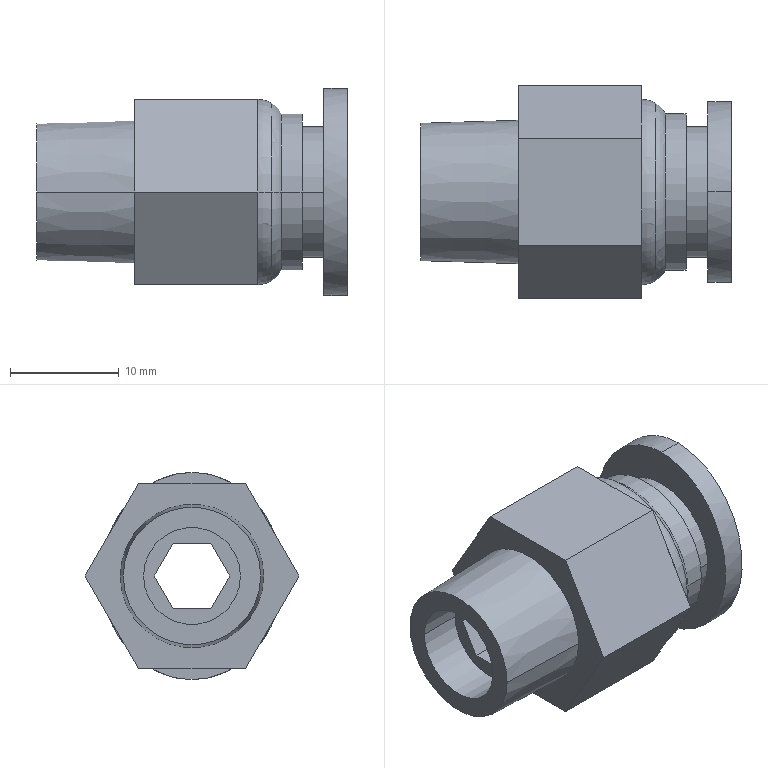Part | Creo | 1 solid | 45 faces | box 28.5 x 19.63 x 19 mm | volume 3530 mm3 | plane 25 | cylinder 8 | torus 8 | cone 2 | other 2 | commonest cylinder face diameters 8.9 x2 10 x2 12 x2 14.36 x2
STEP:
#1=CARTESIAN_POINT('',(308.,140.545,-32.491));
#2=VERTEX_POINT('',#1);
#3=CARTESIAN_POINT('',(308.,149.445,-32.491));
#4=VERTEX_POINT('',#3);
#5=CARTESIAN_POINT('',(308.,144.995,-32.491));
#6=DIRECTION('',(-1.,0.,0.));
#7=DIRECTION('',(0.,-1.,0.));
#8=AXIS2_PLACEMENT_3D('',#5,#6,#7);
#9=CIRCLE('',#8,4.45);
#10=EDGE_CURVE('',#2,#4,#9,.T.);
#11=ORIENTED_EDGE('',*,*,#10,.F.);
#12=CARTESIAN_POINT('',(308.,144.995,-32.491));
#13=DIRECTION('',(-1.,0.,0.));
#14=DIRECTION('',(0.,1.,0.));
#15=AXIS2_PLACEMENT_3D('',#12,#13,#14);
#16=CIRCLE('',#15,4.45);
#17=EDGE_CURVE('',#4,#2,#16,.T.);
#18=ORIENTED_EDGE('',*,*,#17,.F.);
#19=EDGE_LOOP('',(#11,#18));
#20=FACE_OUTER_BOUND('',#19,.F.);
#21=CARTESIAN_POINT('',(308.,146.727,-35.491));
#22=VERTEX_POINT('',#21);
#23=CARTESIAN_POINT('',(308.,148.459,-32.491));
#24=VERTEX_POINT('',#23);
#25=CARTESIAN_POINT('',(308.,146.727,-35.491));
#26=DIRECTION('',(0.,0.5,0.866));
#27=VECTOR('',#26,3.464);
#28=LINE('',#25,#27);
#29=EDGE_CURVE('',#22,#24,#28,.T.);
#30=ORIENTED_EDGE('',*,*,#29,.F.);
#31=CARTESIAN_POINT('',(308.,143.263,-35.491));
#32=VERTEX_POINT('',#31);
#33=CARTESIAN_POINT('',(308.,143.263,-35.491));
#34=DIRECTION('',(0.,1.,0.));
#35=VECTOR('',#34,3.464);
#36=LINE('',#33,#35);
#37=EDGE_CURVE('',#32,#22,#36,.T.);
#38=ORIENTED_EDGE('',*,*,#37,.F.);
#39=CARTESIAN_POINT('',(308.,141.531,-32.491));
#40=VERTEX_POINT('',#39);
#41=CARTESIAN_POINT('',(308.,141.531,-32.491));
#42=DIRECTION('',(0.,0.5,-0.866));
#43=VECTOR('',#42,3.464);
#44=LINE('',#41,#43);
#45=EDGE_CURVE('',#40,#32,#44,.T.);
#46=ORIENTED_EDGE('',*,*,#45,.F.);
#47=CARTESIAN_POINT('',(308.,143.263,-29.491));
#48=VERTEX_POINT('',#47);
#49=CARTESIAN_POINT('',(308.,143.263,-29.491));
#50=DIRECTION('',(0.,-0.5,-0.866));
#51=VECTOR('',#50,3.464);
#52=LINE('',#49,#51);
#53=EDGE_CURVE('',#48,#40,#52,.T.);
#54=ORIENTED_EDGE('',*,*,#53,.F.);
#55=CARTESIAN_POINT('',(308.,146.727,-29.491));
#56=VERTEX_POINT('',#55);
#57=CARTESIAN_POINT('',(308.,146.727,-29.491));
#58=DIRECTION('',(0.,-1.,0.));
#59=VECTOR('',#58,3.464);
#60=LINE('',#57,#59);
#61=EDGE_CURVE('',#56,#48,#60,.T.);
#62=ORIENTED_EDGE('',*,*,#61,.F.);
#63=CARTESIAN_POINT('',(308.,148.459,-32.491));
#64=DIRECTION('',(0.,-0.5,0.866));
#65=VECTOR('',#64,3.464);
#66=LINE('',#63,#65);
#67=EDGE_CURVE('',#24,#56,#66,.T.);
#68=ORIENTED_EDGE('',*,*,#67,.F.);
#69=EDGE_LOOP('',(#30,#38,#46,#54,#62,#68));
#70=FACE_BOUND('',#69,.F.);
#71=CARTESIAN_POINT('',(308.,144.995,-28.041));
#72=DIRECTION('',(1.,0.,0.));
#73=DIRECTION('',(0.,1.,0.));
#74=AXIS2_PLACEMENT_3D('',#71,#72,#73);
#75=PLANE('',#74);
#76=ADVANCED_FACE('',(#20,#70),#75,.F.);
#77=CARTESIAN_POINT('',(304.,149.445,-32.491));
#78=VERTEX_POINT('',#77);
#79=CARTESIAN_POINT('',(304.,140.545,-32.491));
#80=VERTEX_POINT('',#79);
#81=CARTESIAN_POINT('',(304.,144.995,-32.491));
#82=DIRECTION('',(1.,0.,0.));
#83=DIRECTION('',(0.,1.,0.));
#84=AXIS2_PLACEMENT_3D('',#81,#82,#83);
#85=CIRCLE('',#84,4.45);
#86=EDGE_CURVE('',#78,#80,#85,.T.);
#87=ORIENTED_EDGE('',*,*,#86,.T.);
#88=CARTESIAN_POINT('',(308.,140.545,-32.491));
#89=DIRECTION('',(-1.,0.,0.));
#90=VECTOR('',#89,4.);
#91=LINE('',#88,#90);
#92=EDGE_CURVE('',#2,#80,#91,.T.);
#93=ORIENTED_EDGE('',*,*,#92,.F.);
#94=ORIENTED_EDGE('',*,*,#10,.T.);
#95=CARTESIAN_POINT('',(308.,149.445,-32.491));
#96=DIRECTION('',(-1.,0.,0.));
#97=VECTOR('',#96,4.);
#98=LINE('',#95,#97);
#99=EDGE_CURVE('',#4,#78,#98,.T.);
#100=ORIENTED_EDGE('',*,*,#99,.T.);
#101=EDGE_LOOP('',(#87,#93,#94,#100));
#102=FACE_OUTER_BOUND('',#101,.F.);
#103=CARTESIAN_POINT('',(335.,144.995,-32.491));
#104=DIRECTION('',(-1.,0.,0.));
#105=DIRECTION('',(0.,-1.,0.));
#106=AXIS2_PLACEMENT_3D('',#103,#104,#105);
#107=CYLINDRICAL_SURFACE('',#106,4.45);
#108=ADVANCED_FACE('',(#102),#107,.F.);
#109=CARTESIAN_POINT('',(304.,151.296,-32.491));
#110=VERTEX_POINT('',#109);
#111=CARTESIAN_POINT('',(304.,138.694,-32.491));
#112=VERTEX_POINT('',#111);
#113=CARTESIAN_POINT('',(304.,144.995,-32.491));
#114=DIRECTION('',(-1.,0.,0.));
#115=DIRECTION('',(0.,1.,0.));
#116=AXIS2_PLACEMENT_3D('',#113,#114,#115);
#117=CIRCLE('',#116,6.301);
#118=EDGE_CURVE('',#110,#112,#117,.T.);
#119=ORIENTED_EDGE('',*,*,#118,.F.);
#120=CARTESIAN_POINT('',(304.,144.995,-32.491));
#121=DIRECTION('',(-1.,0.,0.));
#122=DIRECTION('',(0.,-1.,0.));
#123=AXIS2_PLACEMENT_3D('',#120,#121,#122);
#124=CIRCLE('',#123,6.301);
#125=EDGE_CURVE('',#112,#110,#124,.T.);
#126=ORIENTED_EDGE('',*,*,#125,.F.);
#127=EDGE_LOOP('',(#119,#126));
#128=FACE_OUTER_BOUND('',#127,.F.);
#129=CARTESIAN_POINT('',(304.,144.995,-32.491));
#130=DIRECTION('',(1.,0.,0.));
#131=DIRECTION('',(0.,-1.,0.));
#132=AXIS2_PLACEMENT_3D('',#129,#130,#131);
#133=CIRCLE('',#132,4.45);
#134=EDGE_CURVE('',#80,#78,#133,.T.);
#135=ORIENTED_EDGE('',*,*,#134,.F.);
#136=ORIENTED_EDGE('',*,*,#86,.F.);
#137=EDGE_LOOP('',(#135,#136));
#138=FACE_BOUND('',#137,.F.);
#139=CARTESIAN_POINT('',(304.,144.995,-26.19));
#140=DIRECTION('',(-1.,0.,0.));
#141=DIRECTION('',(0.,-1.,0.));
#142=AXIS2_PLACEMENT_3D('',#139,#140,#141);
#143=PLANE('',#142);
#144=ADVANCED_FACE('',(#128,#138),#143,.T.);
#145=ORIENTED_EDGE('',*,*,#134,.T.);
#146=ORIENTED_EDGE('',*,*,#99,.F.);
#147=ORIENTED_EDGE('',*,*,#17,.T.);
#148=ORIENTED_EDGE('',*,*,#92,.T.);
#149=EDGE_LOOP('',(#145,#146,#147,#148));
#150=FACE_OUTER_BOUND('',#149,.F.);
#151=CARTESIAN_POINT('',(335.,144.995,-32.491));
#152=DIRECTION('',(-1.,0.,0.));
#153=DIRECTION('',(0.,-1.,0.));
#154=AXIS2_PLACEMENT_3D('',#151,#152,#153);
#155=CYLINDRICAL_SURFACE('',#154,4.45);
#156=ADVANCED_FACE('',(#150),#155,.F.);
#157=ORIENTED_EDGE('',*,*,#118,.T.);
#158=CARTESIAN_POINT('',(313.,138.415,-32.491));
#159=VERTEX_POINT('',#158);
#160=CARTESIAN_POINT('',(304.,138.694,-32.491));
#161=DIRECTION('',(0.9995,-0.03097,0.));
#162=VECTOR('',#161,9.004);
#163=LINE('',#160,#162);
#164=EDGE_CURVE('',#112,#159,#163,.T.);
#165=ORIENTED_EDGE('',*,*,#164,.T.);
#166=CARTESIAN_POINT('',(313.,151.575,-32.491));
#167=VERTEX_POINT('',#166);
#168=CARTESIAN_POINT('',(313.,144.995,-32.491));
#169=DIRECTION('',(1.,0.,0.));
#170=DIRECTION('',(0.,-1.,0.));
#171=AXIS2_PLACEMENT_3D('',#168,#169,#170);
#172=CIRCLE('',#171,6.58);
#173=EDGE_CURVE('',#159,#167,#172,.T.);
#174=ORIENTED_EDGE('',*,*,#173,.T.);
#175=CARTESIAN_POINT('',(304.,151.296,-32.491));
#176=DIRECTION('',(0.9995,0.03097,0.));
#177=VECTOR('',#176,9.004);
#178=LINE('',#175,#177);
#179=EDGE_CURVE('',#110,#167,#178,.T.);
#180=ORIENTED_EDGE('',*,*,#179,.F.);
#181=EDGE_LOOP('',(#157,#165,#174,#180));
#182=FACE_OUTER_BOUND('',#181,.F.);
#183=CARTESIAN_POINT('',(308.5,144.995,-32.491));
#184=DIRECTION('',(1.,0.,0.));
#185=DIRECTION('',(0.,1.,0.));
#186=AXIS2_PLACEMENT_3D('',#183,#184,#185);
#187=CONICAL_SURFACE('',#186,6.441,1.775);
#188=ADVANCED_FACE('',(#182),#187,.T.);
#189=ORIENTED_EDGE('',*,*,#125,.T.);
#190=ORIENTED_EDGE('',*,*,#179,.T.);
#191=CARTESIAN_POINT('',(313.,144.995,-32.491));
#192=DIRECTION('',(1.,0.,0.));
#193=DIRECTION('',(0.,1.,0.));
#194=AXIS2_PLACEMENT_3D('',#191,#192,#193);
#195=CIRCLE('',#194,6.58);
#196=EDGE_CURVE('',#167,#159,#195,.T.);
#197=ORIENTED_EDGE('',*,*,#196,.T.);
#198=ORIENTED_EDGE('',*,*,#164,.F.);
#199=EDGE_LOOP('',(#189,#190,#197,#198));
#200=FACE_OUTER_BOUND('',#199,.F.);
#201=CARTESIAN_POINT('',(308.5,144.995,-32.491));
#202=DIRECTION('',(1.,0.,0.));
#203=DIRECTION('',(0.,1.,0.));
#204=AXIS2_PLACEMENT_3D('',#201,#202,#203);
#205=CONICAL_SURFACE('',#204,6.441,1.775);
#206=ADVANCED_FACE('',(#200),#205,.T.);
#207=CARTESIAN_POINT('',(313.,135.18,-32.491));
#208=VERTEX_POINT('',#207);
#209=CARTESIAN_POINT('',(313.,140.088,-23.991));
#210=VERTEX_POINT('',#209);
#211=CARTESIAN_POINT('',(313.,135.18,-32.491));
#212=DIRECTION('',(0.,0.5,0.866));
#213=VECTOR('',#212,9.815);
#214=LINE('',#211,#213);
#215=EDGE_CURVE('',#208,#210,#214,.T.);
#216=ORIENTED_EDGE('',*,*,#215,.F.);
#217=CARTESIAN_POINT('',(313.,140.088,-40.991));
#218=VERTEX_POINT('',#217);
#219=CARTESIAN_POINT('',(313.,140.088,-40.991));
#220=DIRECTION('',(0.,-0.5,0.866));
#221=VECTOR('',#220,9.815);
#222=LINE('',#219,#221);
#223=EDGE_CURVE('',#218,#208,#222,.T.);
#224=ORIENTED_EDGE('',*,*,#223,.F.);
#225=CARTESIAN_POINT('',(313.,149.903,-40.991));
#226=VERTEX_POINT('',#225);
#227=CARTESIAN_POINT('',(313.,140.088,-40.991));
#228=DIRECTION('',(0.,1.,0.));
#229=VECTOR('',#228,9.815);
#230=LINE('',#227,#229);
#231=EDGE_CURVE('',#218,#226,#230,.T.);
#232=ORIENTED_EDGE('',*,*,#231,.T.);
#233=CARTESIAN_POINT('',(313.,154.81,-32.491));
#234=VERTEX_POINT('',#233);
#235=CARTESIAN_POINT('',(313.,154.81,-32.491));
#236=DIRECTION('',(0.,-0.5,-0.866));
#237=VECTOR('',#236,9.815);
#238=LINE('',#235,#237);
#239=EDGE_CURVE('',#234,#226,#238,.T.);
#240=ORIENTED_EDGE('',*,*,#239,.F.);
#241=CARTESIAN_POINT('',(313.,149.903,-23.991));
#242=VERTEX_POINT('',#241);
#243=CARTESIAN_POINT('',(313.,149.903,-23.991));
#244=DIRECTION('',(0.,0.5,-0.866));
#245=VECTOR('',#244,9.815);
#246=LINE('',#243,#245);
#247=EDGE_CURVE('',#242,#234,#246,.T.);
#248=ORIENTED_EDGE('',*,*,#247,.F.);
#249=CARTESIAN_POINT('',(313.,149.903,-23.991));
#250=DIRECTION('',(0.,-1.,0.));
#251=VECTOR('',#250,9.815);
#252=LINE('',#249,#251);
#253=EDGE_CURVE('',#242,#210,#252,.T.);
#254=ORIENTED_EDGE('',*,*,#253,.T.);
#255=EDGE_LOOP('',(#216,#224,#232,#240,#248,#254));
#256=FACE_OUTER_BOUND('',#255,.F.);
#257=ORIENTED_EDGE('',*,*,#196,.F.);
#258=ORIENTED_EDGE('',*,*,#173,.F.);
#259=EDGE_LOOP('',(#257,#258));
#260=FACE_BOUND('',#259,.F.);
#261=CARTESIAN_POINT('',(313.,144.995,-25.841));
#262=DIRECTION('',(-1.,0.,0.));
#263=DIRECTION('',(0.,-1.,0.));
#264=AXIS2_PLACEMENT_3D('',#261,#262,#263);
#265=PLANE('',#264);
#266=ADVANCED_FACE('',(#256,#260),#265,.T.);
#267=ORIENTED_EDGE('',*,*,#215,.T.);
#268=CARTESIAN_POINT('',(324.3,140.088,-23.991));
#269=VERTEX_POINT('',#268);
#270=CARTESIAN_POINT('',(313.,140.088,-23.991));
#271=DIRECTION('',(1.,0.,0.));
#272=VECTOR('',#271,11.3);
#273=LINE('',#270,#272);
#274=EDGE_CURVE('',#210,#269,#273,.T.);
#275=ORIENTED_EDGE('',*,*,#274,.T.);
#276=CARTESIAN_POINT('',(324.3,137.634,-28.241));
#277=VERTEX_POINT('',#276);
#278=CARTESIAN_POINT('',(324.3,140.088,-23.991));
#279=DIRECTION('',(0.,-0.5,-0.866));
#280=VECTOR('',#279,4.907);
#281=LINE('',#278,#280);
#282=EDGE_CURVE('',#269,#277,#281,.T.);
#283=ORIENTED_EDGE('',*,*,#282,.T.);
#284=CARTESIAN_POINT('',(324.3,135.18,-32.491));
#285=VERTEX_POINT('',#284);
#286=CARTESIAN_POINT('',(324.3,137.634,-28.241));
#287=DIRECTION('',(0.,-0.5,-0.866));
#288=VECTOR('',#287,4.907);
#289=LINE('',#286,#288);
#290=EDGE_CURVE('',#277,#285,#289,.T.);
#291=ORIENTED_EDGE('',*,*,#290,.T.);
#292=CARTESIAN_POINT('',(313.,135.18,-32.491));
#293=DIRECTION('',(1.,0.,0.));
#294=VECTOR('',#293,11.3);
#295=LINE('',#292,#294);
#296=EDGE_CURVE('',#208,#285,#295,.T.);
#297=ORIENTED_EDGE('',*,*,#296,.F.);
#298=EDGE_LOOP('',(#267,#275,#283,#291,#297));
#299=FACE_OUTER_BOUND('',#298,.F.);
#300=CARTESIAN_POINT('',(324.3,135.18,-32.491));
#301=DIRECTION('',(0.,-0.866,0.5));
#302=DIRECTION('',(0.,-0.5,-0.866));
#303=AXIS2_PLACEMENT_3D('',#300,#301,#302);
#304=PLANE('',#303);
#305=ADVANCED_FACE('',(#299),#304,.T.);
#306=ORIENTED_EDGE('',*,*,#253,.F.);
#307=CARTESIAN_POINT('',(324.3,149.903,-23.991));
#308=VERTEX_POINT('',#307);
#309=CARTESIAN_POINT('',(313.,149.903,-23.991));
#310=DIRECTION('',(1.,0.,0.));
#311=VECTOR('',#310,11.3);
#312=LINE('',#309,#311);
#313=EDGE_CURVE('',#242,#308,#312,.T.);
#314=ORIENTED_EDGE('',*,*,#313,.T.);
#315=CARTESIAN_POINT('',(324.3,144.995,-23.991));
#316=VERTEX_POINT('',#315);
#317=CARTESIAN_POINT('',(324.3,149.903,-23.991));
#318=DIRECTION('',(0.,-1.,0.));
#319=VECTOR('',#318,4.907);
#320=LINE('',#317,#319);
#321=EDGE_CURVE('',#308,#316,#320,.T.);
#322=ORIENTED_EDGE('',*,*,#321,.T.);
#323=CARTESIAN_POINT('',(324.3,144.995,-23.991));
#324=DIRECTION('',(0.,-1.,0.));
#325=VECTOR('',#324,4.907);
#326=LINE('',#323,#325);
#327=EDGE_CURVE('',#316,#269,#326,.T.);
#328=ORIENTED_EDGE('',*,*,#327,.T.);
#329=ORIENTED_EDGE('',*,*,#274,.F.);
#330=EDGE_LOOP('',(#306,#314,#322,#328,#329));
#331=FACE_OUTER_BOUND('',#330,.F.);
#332=CARTESIAN_POINT('',(324.3,140.088,-23.991));
#333=DIRECTION('',(0.,0.,1.));
#334=DIRECTION('',(1.,0.,0.));
#335=AXIS2_PLACEMENT_3D('',#332,#333,#334);
#336=PLANE('',#335);
#337=ADVANCED_FACE('',(#331),#336,.T.);
#338=CARTESIAN_POINT('',(324.3,154.81,-32.491));
#339=VERTEX_POINT('',#338);
#340=CARTESIAN_POINT('',(313.,154.81,-32.491));
#341=DIRECTION('',(1.,0.,0.));
#342=VECTOR('',#341,11.3);
#343=LINE('',#340,#342);
#344=EDGE_CURVE('',#234,#339,#343,.T.);
#345=ORIENTED_EDGE('',*,*,#344,.T.);
#346=CARTESIAN_POINT('',(324.3,152.357,-28.241));
#347=VERTEX_POINT('',#346);
#348=CARTESIAN_POINT('',(324.3,154.81,-32.491));
#349=DIRECTION('',(0.,-0.5,0.866));
#350=VECTOR('',#349,4.907);
#351=LINE('',#348,#350);
#352=EDGE_CURVE('',#339,#347,#351,.T.);
#353=ORIENTED_EDGE('',*,*,#352,.T.);
#354=CARTESIAN_POINT('',(324.3,152.357,-28.241));
#355=DIRECTION('',(0.,-0.5,0.866));
#356=VECTOR('',#355,4.907);
#357=LINE('',#354,#356);
#358=EDGE_CURVE('',#347,#308,#357,.T.);
#359=ORIENTED_EDGE('',*,*,#358,.T.);
#360=ORIENTED_EDGE('',*,*,#313,.F.);
#361=ORIENTED_EDGE('',*,*,#247,.T.);
#362=EDGE_LOOP('',(#345,#353,#359,#360,#361));
#363=FACE_OUTER_BOUND('',#362,.F.);
#364=CARTESIAN_POINT('',(324.3,149.903,-23.991));
#365=DIRECTION('',(0.,0.866,0.5));
#366=DIRECTION('',(0.,-0.5,0.866));
#367=AXIS2_PLACEMENT_3D('',#364,#365,#366);
#368=PLANE('',#367);
#369=ADVANCED_FACE('',(#363),#368,.T.);
#370=ORIENTED_EDGE('',*,*,#239,.T.);
#371=CARTESIAN_POINT('',(324.3,149.903,-40.991));
#372=VERTEX_POINT('',#371);
#373=CARTESIAN_POINT('',(313.,149.903,-40.991));
#374=DIRECTION('',(1.,0.,0.));
#375=VECTOR('',#374,11.3);
#376=LINE('',#373,#375);
#377=EDGE_CURVE('',#226,#372,#376,.T.);
#378=ORIENTED_EDGE('',*,*,#377,.T.);
#379=CARTESIAN_POINT('',(324.3,152.357,-36.741));
#380=VERTEX_POINT('',#379);
#381=CARTESIAN_POINT('',(324.3,149.903,-40.991));
#382=DIRECTION('',(0.,0.5,0.866));
#383=VECTOR('',#382,4.907);
#384=LINE('',#381,#383);
#385=EDGE_CURVE('',#372,#380,#384,.T.);
#386=ORIENTED_EDGE('',*,*,#385,.T.);
#387=CARTESIAN_POINT('',(324.3,152.357,-36.741));
#388=DIRECTION('',(0.,0.5,0.866));
#389=VECTOR('',#388,4.907);
#390=LINE('',#387,#389);
#391=EDGE_CURVE('',#380,#339,#390,.T.);
#392=ORIENTED_EDGE('',*,*,#391,.T.);
#393=ORIENTED_EDGE('',*,*,#344,.F.);
#394=EDGE_LOOP('',(#370,#378,#386,#392,#393));
#395=FACE_OUTER_BOUND('',#394,.F.);
#396=CARTESIAN_POINT('',(324.3,154.81,-32.491));
#397=DIRECTION('',(0.,0.866,-0.5));
#398=DIRECTION('',(0.,0.5,0.866));
#399=AXIS2_PLACEMENT_3D('',#396,#397,#398);
#400=PLANE('',#399);
#401=ADVANCED_FACE('',(#395),#400,.T.);
#402=ORIENTED_EDGE('',*,*,#231,.F.);
#403=CARTESIAN_POINT('',(324.3,140.088,-40.991));
#404=VERTEX_POINT('',#403);
#405=CARTESIAN_POINT('',(313.,140.088,-40.991));
#406=DIRECTION('',(1.,0.,0.));
#407=VECTOR('',#406,11.3);
#408=LINE('',#405,#407);
#409=EDGE_CURVE('',#218,#404,#408,.T.);
#410=ORIENTED_EDGE('',*,*,#409,.T.);
#411=CARTESIAN_POINT('',(324.3,144.995,-40.991));
#412=VERTEX_POINT('',#411);
#413=CARTESIAN_POINT('',(324.3,140.088,-40.991));
#414=DIRECTION('',(0.,1.,0.));
#415=VECTOR('',#414,4.907);
#416=LINE('',#413,#415);
#417=EDGE_CURVE('',#404,#412,#416,.T.);
#418=ORIENTED_EDGE('',*,*,#417,.T.);
#419=CARTESIAN_POINT('',(324.3,144.995,-40.991));
#420=DIRECTION('',(0.,1.,0.));
#421=VECTOR('',#420,4.907);
#422=LINE('',#419,#421);
#423=EDGE_CURVE('',#412,#372,#422,.T.);
#424=ORIENTED_EDGE('',*,*,#423,.T.);
#425=ORIENTED_EDGE('',*,*,#377,.F.);
#426=EDGE_LOOP('',(#402,#410,#418,#424,#425));
#427=FACE_OUTER_BOUND('',#426,.F.);
#428=CARTESIAN_POINT('',(324.3,149.903,-40.991));
#429=DIRECTION('',(0.,0.,-1.));
#430=DIRECTION('',(0.,1.,0.));
#431=AXIS2_PLACEMENT_3D('',#428,#429,#430);
#432=PLANE('',#431);
#433=ADVANCED_FACE('',(#427),#432,.T.);
#434=ORIENTED_EDGE('',*,*,#223,.T.);
#435=ORIENTED_EDGE('',*,*,#296,.T.);
#436=CARTESIAN_POINT('',(324.3,137.634,-36.741));
#437=VERTEX_POINT('',#436);
#438=CARTESIAN_POINT('',(324.3,135.18,-32.491));
#439=DIRECTION('',(0.,0.5,-0.866));
#440=VECTOR('',#439,4.907);
#441=LINE('',#438,#440);
#442=EDGE_CURVE('',#285,#437,#441,.T.);
#443=ORIENTED_EDGE('',*,*,#442,.T.);
#444=CARTESIAN_POINT('',(324.3,137.634,-36.741));
#445=DIRECTION('',(0.,0.5,-0.866));
#446=VECTOR('',#445,4.907);
#447=LINE('',#444,#446);
#448=EDGE_CURVE('',#437,#404,#447,.T.);
#449=ORIENTED_EDGE('',*,*,#448,.T.);
#450=ORIENTED_EDGE('',*,*,#409,.F.);
#451=EDGE_LOOP('',(#434,#435,#443,#449,#450));
#452=FACE_OUTER_BOUND('',#451,.F.);
#453=CARTESIAN_POINT('',(324.3,140.088,-40.991));
#454=DIRECTION('',(0.,-0.866,-0.5));
#455=DIRECTION('',(0.,0.5,-0.866));
#456=AXIS2_PLACEMENT_3D('',#453,#454,#455);
#457=PLANE('',#456);
#458=ADVANCED_FACE('',(#452),#457,.T.);
#459=CARTESIAN_POINT('',(324.3,136.495,-32.491));
#460=VERTEX_POINT('',#459);
#461=CARTESIAN_POINT('',(324.3,144.995,-32.491));
#462=DIRECTION('',(-1.,0.,0.));
#463=DIRECTION('',(0.,-0.866,-0.5));
#464=AXIS2_PLACEMENT_3D('',#461,#462,#463);
#465=CIRCLE('',#464,8.5);
#466=EDGE_CURVE('',#437,#460,#465,.T.);
#467=ORIENTED_EDGE('',*,*,#466,.F.);
#468=ORIENTED_EDGE('',*,*,#442,.F.);
#469=ORIENTED_EDGE('',*,*,#290,.F.);
#470=CARTESIAN_POINT('',(324.3,144.995,-32.491));
#471=DIRECTION('',(-1.,0.,0.));
#472=DIRECTION('',(0.,-1.,0.));
#473=AXIS2_PLACEMENT_3D('',#470,#471,#472);
#474=CIRCLE('',#473,8.5);
#475=EDGE_CURVE('',#460,#277,#474,.T.);
#476=ORIENTED_EDGE('',*,*,#475,.F.);
#477=EDGE_LOOP('',(#467,#468,#469,#476));
#478=FACE_OUTER_BOUND('',#477,.F.);
#479=CARTESIAN_POINT('',(324.3,144.995,-32.491));
#480=DIRECTION('',(-1.,0.,0.));
#481=DIRECTION('',(0.,-1.,0.));
#482=AXIS2_PLACEMENT_3D('',#479,#480,#481);
#483=PLANE('',#482);
#484=ADVANCED_FACE('',(#478),#483,.F.);
#485=ORIENTED_EDGE('',*,*,#466,.T.);
#486=CARTESIAN_POINT('',(325.561,136.852,-32.491));
#487=VERTEX_POINT('',#486);
#488=CARTESIAN_POINT('',(324.3,138.906,-32.491));
#489=DIRECTION('',(0.,0.,1.));
#490=DIRECTION('',(0.,-1.,0.));
#491=AXIS2_PLACEMENT_3D('',#488,#489,#490);
#492=CIRCLE('',#491,2.411);
#493=EDGE_CURVE('',#460,#487,#492,.T.);
#494=ORIENTED_EDGE('',*,*,#493,.T.);
#495=CARTESIAN_POINT('',(325.561,153.139,-32.491));
#496=VERTEX_POINT('',#495);
#497=CARTESIAN_POINT('',(325.561,144.995,-32.491));
#498=DIRECTION('',(1.,0.,0.));
#499=DIRECTION('',(0.,-1.,0.));
#500=AXIS2_PLACEMENT_3D('',#497,#498,#499);
#501=CIRCLE('',#500,8.144);
#502=EDGE_CURVE('',#487,#496,#501,.T.);
#503=ORIENTED_EDGE('',*,*,#502,.T.);
#504=CARTESIAN_POINT('',(324.3,153.495,-32.491));
#505=VERTEX_POINT('',#504);
#506=CARTESIAN_POINT('',(324.3,151.084,-32.491));
#507=DIRECTION('',(0.,0.,-1.));
#508=DIRECTION('',(0.,1.,0.));
#509=AXIS2_PLACEMENT_3D('',#506,#507,#508);
#510=CIRCLE('',#509,2.411);
#511=EDGE_CURVE('',#505,#496,#510,.T.);
#512=ORIENTED_EDGE('',*,*,#511,.F.);
#513=CARTESIAN_POINT('',(324.3,144.995,-32.491));
#514=DIRECTION('',(-1.,0.,0.));
#515=DIRECTION('',(0.,1.,0.));
#516=AXIS2_PLACEMENT_3D('',#513,#514,#515);
#517=CIRCLE('',#516,8.5);
#518=EDGE_CURVE('',#505,#380,#517,.T.);
#519=ORIENTED_EDGE('',*,*,#518,.T.);
#520=CARTESIAN_POINT('',(324.3,144.995,-32.491));
#521=DIRECTION('',(-1.,0.,0.));
#522=DIRECTION('',(0.,0.866,-0.5));
#523=AXIS2_PLACEMENT_3D('',#520,#521,#522);
#524=CIRCLE('',#523,8.5);
#525=EDGE_CURVE('',#380,#412,#524,.T.);
#526=ORIENTED_EDGE('',*,*,#525,.T.);
#527=CARTESIAN_POINT('',(324.3,144.995,-32.491));
#528=DIRECTION('',(-1.,0.,0.));
#529=DIRECTION('',(0.,0.,-1.));
#530=AXIS2_PLACEMENT_3D('',#527,#528,#529);
#531=CIRCLE('',#530,8.5);
#532=EDGE_CURVE('',#412,#437,#531,.T.);
#533=ORIENTED_EDGE('',*,*,#532,.T.);
#534=EDGE_LOOP('',(#485,#494,#503,#512,#519,#526,#533));
#535=FACE_OUTER_BOUND('',#534,.F.);
#536=CARTESIAN_POINT('',(324.3,144.995,-32.491));
#537=DIRECTION('',(1.,0.,0.));
#538=DIRECTION('',(0.,1.,0.));
#539=AXIS2_PLACEMENT_3D('',#536,#537,#538);
#540=TOROIDAL_SURFACE('',#539,6.089,2.411);
#541=ADVANCED_FACE('',(#535),#540,.T.);
#542=CARTESIAN_POINT('',(324.3,144.995,-32.491));
#543=DIRECTION('',(-1.,0.,0.));
#544=DIRECTION('',(0.,0.,1.));
#545=AXIS2_PLACEMENT_3D('',#542,#543,#544);
#546=CIRCLE('',#545,8.5);
#547=EDGE_CURVE('',#316,#347,#546,.T.);
#548=ORIENTED_EDGE('',*,*,#547,.T.);
#549=CARTESIAN_POINT('',(324.3,144.995,-32.491));
#550=DIRECTION('',(-1.,0.,0.));
#551=DIRECTION('',(0.,0.866,0.5));
#552=AXIS2_PLACEMENT_3D('',#549,#550,#551);
#553=CIRCLE('',#552,8.5);
#554=EDGE_CURVE('',#347,#505,#553,.T.);
#555=ORIENTED_EDGE('',*,*,#554,.T.);
#556=ORIENTED_EDGE('',*,*,#511,.T.);
#557=CARTESIAN_POINT('',(325.561,144.995,-32.491));
#558=DIRECTION('',(1.,0.,0.));
#559=DIRECTION('',(0.,1.,0.));
#560=AXIS2_PLACEMENT_3D('',#557,#558,#559);
#561=CIRCLE('',#560,8.144);
#562=EDGE_CURVE('',#496,#487,#561,.T.);
#563=ORIENTED_EDGE('',*,*,#562,.T.);
#564=ORIENTED_EDGE('',*,*,#493,.F.);
#565=ORIENTED_EDGE('',*,*,#475,.T.);
#566=CARTESIAN_POINT('',(324.3,144.995,-32.491));
#567=DIRECTION('',(-1.,0.,0.));
#568=DIRECTION('',(0.,-0.866,0.5));
#569=AXIS2_PLACEMENT_3D('',#566,#567,#568);
#570=CIRCLE('',#569,8.5);
#571=EDGE_CURVE('',#277,#316,#570,.T.);
#572=ORIENTED_EDGE('',*,*,#571,.T.);
#573=EDGE_LOOP('',(#548,#555,#556,#563,#564,#565,#572));
#574=FACE_OUTER_BOUND('',#573,.F.);
#575=CARTESIAN_POINT('',(324.3,144.995,-32.491));
#576=DIRECTION('',(1.,0.,0.));
#577=DIRECTION('',(0.,1.,0.));
#578=AXIS2_PLACEMENT_3D('',#575,#576,#577);
#579=TOROIDAL_SURFACE('',#578,6.089,2.411);
#580=ADVANCED_FACE('',(#574),#579,.T.);
#581=ORIENTED_EDGE('',*,*,#547,.F.);
#582=ORIENTED_EDGE('',*,*,#321,.F.);
#583=ORIENTED_EDGE('',*,*,#358,.F.);
#584=EDGE_LOOP('',(#581,#582,#583));
#585=FACE_OUTER_BOUND('',#584,.F.);
#586=CARTESIAN_POINT('',(324.3,144.995,-32.491));
#587=DIRECTION('',(-1.,0.,0.));
#588=DIRECTION('',(0.,-1.,0.));
#589=AXIS2_PLACEMENT_3D('',#586,#587,#588);
#590=PLANE('',#589);
#591=ADVANCED_FACE('',(#585),#590,.F.);
#592=ORIENTED_EDGE('',*,*,#518,.F.);
#593=ORIENTED_EDGE('',*,*,#554,.F.);
#594=ORIENTED_EDGE('',*,*,#352,.F.);
#595=ORIENTED_EDGE('',*,*,#391,.F.);
#596=EDGE_LOOP('',(#592,#593,#594,#595));
#597=FACE_OUTER_BOUND('',#596,.F.);
#598=CARTESIAN_POINT('',(324.3,144.995,-32.491));
#599=DIRECTION('',(-1.,0.,0.));
#600=DIRECTION('',(0.,-1.,0.));
#601=AXIS2_PLACEMENT_3D('',#598,#599,#600);
#602=PLANE('',#601);
#603=ADVANCED_FACE('',(#597),#602,.F.);
#604=CARTESIAN_POINT('',(326.45,137.815,-32.491));
#605=VERTEX_POINT('',#604);
#606=CARTESIAN_POINT('',(326.45,152.175,-32.491));
#607=VERTEX_POINT('',#606);
#608=CARTESIAN_POINT('',(326.45,144.995,-32.491));
#609=DIRECTION('',(-1.,0.,0.));
#610=DIRECTION('',(0.,-1.,0.));
#611=AXIS2_PLACEMENT_3D('',#608,#609,#610);
#612=CIRCLE('',#611,7.18);
#613=EDGE_CURVE('',#605,#607,#612,.T.);
#614=ORIENTED_EDGE('',*,*,#613,.F.);
#615=CARTESIAN_POINT('',(324.3,138.906,-32.491));
#616=DIRECTION('',(0.,0.,1.));
#617=DIRECTION('',(0.5232,-0.8522,0.));
#618=AXIS2_PLACEMENT_3D('',#615,#616,#617);
#619=CIRCLE('',#618,2.411);
#620=EDGE_CURVE('',#487,#605,#619,.T.);
#621=ORIENTED_EDGE('',*,*,#620,.F.);
#622=ORIENTED_EDGE('',*,*,#562,.F.);
#623=CARTESIAN_POINT('',(324.3,151.084,-32.491));
#624=DIRECTION('',(0.,0.,-1.));
#625=DIRECTION('',(0.5232,0.8522,0.));
#626=AXIS2_PLACEMENT_3D('',#623,#624,#625);
#627=CIRCLE('',#626,2.411);
#628=EDGE_CURVE('',#496,#607,#627,.T.);
#629=ORIENTED_EDGE('',*,*,#628,.T.);
#630=EDGE_LOOP('',(#614,#621,#622,#629));
#631=FACE_OUTER_BOUND('',#630,.F.);
#632=CARTESIAN_POINT('',(324.3,144.995,-32.491));
#633=DIRECTION('',(1.,0.,0.));
#634=DIRECTION('',(0.,1.,0.));
#635=AXIS2_PLACEMENT_3D('',#632,#633,#634);
#636=TOROIDAL_SURFACE('',#635,6.089,2.411);
#637=ADVANCED_FACE('',(#631),#636,.T.);
#638=ORIENTED_EDGE('',*,*,#613,.T.);
#639=CARTESIAN_POINT('',(328.35,152.175,-32.491));
#640=VERTEX_POINT('',#639);
#641=CARTESIAN_POINT('',(326.45,152.175,-32.491));
#642=DIRECTION('',(1.,0.,0.));
#643=VECTOR('',#642,1.9);
#644=LINE('',#641,#643);
#645=EDGE_CURVE('',#607,#640,#644,.T.);
#646=ORIENTED_EDGE('',*,*,#645,.T.);
#647=CARTESIAN_POINT('',(328.35,137.815,-32.491));
#648=VERTEX_POINT('',#647);
#649=CARTESIAN_POINT('',(328.35,144.995,-32.491));
#650=DIRECTION('',(1.,0.,0.));
#651=DIRECTION('',(0.,1.,0.));
#652=AXIS2_PLACEMENT_3D('',#649,#650,#651);
#653=CIRCLE('',#652,7.18);
#654=EDGE_CURVE('',#640,#648,#653,.T.);
#655=ORIENTED_EDGE('',*,*,#654,.T.);
#656=CARTESIAN_POINT('',(326.45,137.815,-32.491));
#657=DIRECTION('',(1.,0.,0.));
#658=VECTOR('',#657,1.9);
#659=LINE('',#656,#658);
#660=EDGE_CURVE('',#605,#648,#659,.T.);
#661=ORIENTED_EDGE('',*,*,#660,.F.);
#662=EDGE_LOOP('',(#638,#646,#655,#661));
#663=FACE_OUTER_BOUND('',#662,.F.);
#664=CARTESIAN_POINT('',(335.,144.995,-32.491));
#665=DIRECTION('',(1.,0.,0.));
#666=DIRECTION('',(0.,1.,0.));
#667=AXIS2_PLACEMENT_3D('',#664,#665,#666);
#668=CYLINDRICAL_SURFACE('',#667,7.18);
#669=ADVANCED_FACE('',(#663),#668,.T.);
#670=CARTESIAN_POINT('',(326.45,144.995,-32.491));
#671=DIRECTION('',(-1.,0.,0.));
#672=DIRECTION('',(0.,1.,0.));
#673=AXIS2_PLACEMENT_3D('',#670,#671,#672);
#674=CIRCLE('',#673,7.18);
#675=EDGE_CURVE('',#607,#605,#674,.T.);
#676=ORIENTED_EDGE('',*,*,#675,.T.);
#677=ORIENTED_EDGE('',*,*,#660,.T.);
#678=CARTESIAN_POINT('',(328.35,144.995,-32.491));
#679=DIRECTION('',(1.,0.,0.));
#680=DIRECTION('',(0.,-1.,0.));
#681=AXIS2_PLACEMENT_3D('',#678,#679,#680);
#682=CIRCLE('',#681,7.18);
#683=EDGE_CURVE('',#648,#640,#682,.T.);
#684=ORIENTED_EDGE('',*,*,#683,.T.);
#685=ORIENTED_EDGE('',*,*,#645,.F.);
#686=EDGE_LOOP('',(#676,#677,#684,#685));
#687=FACE_OUTER_BOUND('',#686,.F.);
#688=CARTESIAN_POINT('',(335.,144.995,-32.491));
#689=DIRECTION('',(1.,0.,0.));
#690=DIRECTION('',(0.,1.,0.));
#691=AXIS2_PLACEMENT_3D('',#688,#689,#690);
#692=CYLINDRICAL_SURFACE('',#691,7.18);
#693=ADVANCED_FACE('',(#687),#692,.T.);
#694=ORIENTED_EDGE('',*,*,#675,.F.);
#695=ORIENTED_EDGE('',*,*,#628,.F.);
#696=ORIENTED_EDGE('',*,*,#502,.F.);
#697=ORIENTED_EDGE('',*,*,#620,.T.);
#698=EDGE_LOOP('',(#694,#695,#696,#697));
#699=FACE_OUTER_BOUND('',#698,.F.);
#700=CARTESIAN_POINT('',(324.3,144.995,-32.491));
#701=DIRECTION('',(1.,0.,0.));
#702=DIRECTION('',(0.,1.,0.));
#703=AXIS2_PLACEMENT_3D('',#700,#701,#702);
#704=TOROIDAL_SURFACE('',#703,6.089,2.411);
#705=ADVANCED_FACE('',(#699),#704,.T.);
#706=ORIENTED_EDGE('',*,*,#654,.F.);
#707=ORIENTED_EDGE('',*,*,#683,.F.);
#708=EDGE_LOOP('',(#706,#707));
#709=FACE_OUTER_BOUND('',#708,.F.);
#710=CARTESIAN_POINT('',(328.35,150.995,-32.491));
#711=VERTEX_POINT('',#710);
#712=CARTESIAN_POINT('',(328.35,138.995,-32.491));
#713=VERTEX_POINT('',#712);
#714=CARTESIAN_POINT('',(328.35,144.995,-32.491));
#715=DIRECTION('',(-1.,0.,0.));
#716=DIRECTION('',(0.,1.,0.));
#717=AXIS2_PLACEMENT_3D('',#714,#715,#716);
#718=CIRCLE('',#717,6.);
#719=EDGE_CURVE('',#711,#713,#718,.T.);
#720=ORIENTED_EDGE('',*,*,#719,.F.);
#721=CARTESIAN_POINT('',(328.35,144.995,-32.491));
#722=DIRECTION('',(-1.,0.,0.));
#723=DIRECTION('',(0.,-1.,0.));
#724=AXIS2_PLACEMENT_3D('',#721,#722,#723);
#725=CIRCLE('',#724,6.);
#726=EDGE_CURVE('',#713,#711,#725,.T.);
#727=ORIENTED_EDGE('',*,*,#726,.F.);
#728=EDGE_LOOP('',(#720,#727));
#729=FACE_BOUND('',#728,.F.);
#730=CARTESIAN_POINT('',(328.35,144.995,-26.491));
#731=DIRECTION('',(1.,0.,0.));
#732=DIRECTION('',(0.,1.,0.));
#733=AXIS2_PLACEMENT_3D('',#730,#731,#732);
#734=PLANE('',#733);
#735=ADVANCED_FACE('',(#709,#729),#734,.T.);
#736=ORIENTED_EDGE('',*,*,#719,.T.);
#737=CARTESIAN_POINT('',(330.35,138.995,-32.491));
#738=VERTEX_POINT('',#737);
#739=CARTESIAN_POINT('',(328.35,138.995,-32.491));
#740=DIRECTION('',(1.,0.,0.));
#741=VECTOR('',#740,2.);
#742=LINE('',#739,#741);
#743=EDGE_CURVE('',#713,#738,#742,.T.);
#744=ORIENTED_EDGE('',*,*,#743,.T.);
#745=CARTESIAN_POINT('',(330.35,150.995,-32.491));
#746=VERTEX_POINT('',#745);
#747=CARTESIAN_POINT('',(330.35,144.995,-32.491));
#748=DIRECTION('',(1.,0.,0.));
#749=DIRECTION('',(0.,-1.,0.));
#750=AXIS2_PLACEMENT_3D('',#747,#748,#749);
#751=CIRCLE('',#750,6.);
#752=EDGE_CURVE('',#738,#746,#751,.T.);
#753=ORIENTED_EDGE('',*,*,#752,.T.);
#754=CARTESIAN_POINT('',(328.35,150.995,-32.491));
#755=DIRECTION('',(1.,0.,0.));
#756=VECTOR('',#755,2.);
#757=LINE('',#754,#756);
#758=EDGE_CURVE('',#711,#746,#757,.T.);
#759=ORIENTED_EDGE('',*,*,#758,.F.);
#760=EDGE_LOOP('',(#736,#744,#753,#759));
#761=FACE_OUTER_BOUND('',#760,.F.);
#762=CARTESIAN_POINT('',(335.,144.995,-32.491));
#763=DIRECTION('',(1.,0.,0.));
#764=DIRECTION('',(0.,1.,0.));
#765=AXIS2_PLACEMENT_3D('',#762,#763,#764);
#766=CYLINDRICAL_SURFACE('',#765,6.);
#767=ADVANCED_FACE('',(#761),#766,.T.);
#768=ORIENTED_EDGE('',*,*,#726,.T.);
#769=ORIENTED_EDGE('',*,*,#758,.T.);
#770=CARTESIAN_POINT('',(330.35,144.995,-32.491));
#771=DIRECTION('',(1.,0.,0.));
#772=DIRECTION('',(0.,1.,0.));
#773=AXIS2_PLACEMENT_3D('',#770,#771,#772);
#774=CIRCLE('',#773,6.);
#775=EDGE_CURVE('',#746,#738,#774,.T.);
#776=ORIENTED_EDGE('',*,*,#775,.T.);
#777=ORIENTED_EDGE('',*,*,#743,.F.);
#778=EDGE_LOOP('',(#768,#769,#776,#777));
#779=FACE_OUTER_BOUND('',#778,.F.);
#780=CARTESIAN_POINT('',(335.,144.995,-32.491));
#781=DIRECTION('',(1.,0.,0.));
#782=DIRECTION('',(0.,1.,0.));
#783=AXIS2_PLACEMENT_3D('',#780,#781,#782);
#784=CYLINDRICAL_SURFACE('',#783,6.);
#785=ADVANCED_FACE('',(#779),#784,.T.);
#786=CARTESIAN_POINT('',(330.35,144.995,-22.991));
#787=VERTEX_POINT('',#786);
#788=CARTESIAN_POINT('',(330.35,144.995,-41.991));
#789=VERTEX_POINT('',#788);
#790=CARTESIAN_POINT('',(330.35,144.995,-22.991));
#791=CARTESIAN_POINT('',(330.35,145.484,-22.991));
#792=CARTESIAN_POINT('',(330.35,146.499,-23.09));
#793=CARTESIAN_POINT('',(330.35,148.06,-23.594));
#794=CARTESIAN_POINT('',(330.35,149.564,-24.479));
#795=CARTESIAN_POINT('',(330.35,150.907,-25.725));
#796=CARTESIAN_POINT('',(330.35,151.995,-27.262));
#797=CARTESIAN_POINT('',(330.35,152.768,-28.983));
#798=CARTESIAN_POINT('',(330.35,153.135,-30.471));
#799=CARTESIAN_POINT('',(330.35,153.274,-31.642));
#800=CARTESIAN_POINT('',(330.35,153.306,-32.491));
#801=CARTESIAN_POINT('',(330.35,153.274,-33.34));
#802=CARTESIAN_POINT('',(330.35,153.135,-34.511));
#803=CARTESIAN_POINT('',(330.35,152.768,-35.998));
#804=CARTESIAN_POINT('',(330.35,151.995,-37.72));
#805=CARTESIAN_POINT('',(330.35,150.907,-39.257));
#806=CARTESIAN_POINT('',(330.35,149.564,-40.502));
#807=CARTESIAN_POINT('',(330.35,148.06,-41.387));
#808=CARTESIAN_POINT('',(330.35,146.499,-41.891));
#809=CARTESIAN_POINT('',(330.35,145.484,-41.991));
#810=CARTESIAN_POINT('',(330.35,144.995,-41.991));
#811=B_SPLINE_CURVE_WITH_KNOTS('',3,(#790,#791,#792,#793,#794,#795,#796,#797,#798,#799,#800,#801,#802,#803,#804,#805,#806,#807,#808,#809,#810),.UNSPECIFIED.,.F.,.F.,(4,1,1,1,1,1,1,1,1,1,1,1,1,1,1,1,1,1,4),(0.,0.0625,0.125,0.1875,0.25,0.3125,0.375,0.4375,0.4688,0.5,0.5312,0.5625,0.625,0.6875,0.75,0.8125,0.875,0.9375,1.),.UNSPECIFIED.);
#812=EDGE_CURVE('',#787,#789,#811,.T.);
#813=ORIENTED_EDGE('',*,*,#812,.F.);
#814=CARTESIAN_POINT('',(330.35,144.995,-41.991));
#815=CARTESIAN_POINT('',(330.35,144.506,-41.991));
#816=CARTESIAN_POINT('',(330.35,143.491,-41.891));
#817=CARTESIAN_POINT('',(330.35,141.931,-41.387));
#818=CARTESIAN_POINT('',(330.35,140.427,-40.502));
#819=CARTESIAN_POINT('',(330.35,139.084,-39.257));
#820=CARTESIAN_POINT('',(330.35,137.996,-37.72));
#821=CARTESIAN_POINT('',(330.35,137.223,-35.998));
#822=CARTESIAN_POINT('',(330.35,136.856,-34.511));
#823=CARTESIAN_POINT('',(330.35,136.717,-33.34));
#824=CARTESIAN_POINT('',(330.35,136.684,-32.491));
#825=CARTESIAN_POINT('',(330.35,136.717,-31.642));
#826=CARTESIAN_POINT('',(330.35,136.856,-30.471));
#827=CARTESIAN_POINT('',(330.35,137.223,-28.983));
#828=CARTESIAN_POINT('',(330.35,137.996,-27.262));
#829=CARTESIAN_POINT('',(330.35,139.084,-25.725));
#830=CARTESIAN_POINT('',(330.35,140.427,-24.479));
#831=CARTESIAN_POINT('',(330.35,141.931,-23.594));
#832=CARTESIAN_POINT('',(330.35,143.491,-23.09));
#833=CARTESIAN_POINT('',(330.35,144.506,-22.991));
#834=CARTESIAN_POINT('',(330.35,144.995,-22.991));
#835=B_SPLINE_CURVE_WITH_KNOTS('',3,(#814,#815,#816,#817,#818,#819,#820,#821,#822,#823,#824,#825,#826,#827,#828,#829,#830,#831,#832,#833,#834),.UNSPECIFIED.,.F.,.F.,(4,1,1,1,1,1,1,1,1,1,1,1,1,1,1,1,1,1,4),(0.,0.0625,0.125,0.1875,0.25,0.3125,0.375,0.4375,0.4688,0.5,0.5312,0.5625,0.625,0.6875,0.75,0.8125,0.875,0.9375,1.),.UNSPECIFIED.);
#836=EDGE_CURVE('',#789,#787,#835,.T.);
#837=ORIENTED_EDGE('',*,*,#836,.F.);
#838=EDGE_LOOP('',(#813,#837));
#839=FACE_OUTER_BOUND('',#838,.F.);
#840=ORIENTED_EDGE('',*,*,#775,.F.);
#841=ORIENTED_EDGE('',*,*,#752,.F.);
#842=EDGE_LOOP('',(#840,#841));
#843=FACE_BOUND('',#842,.F.);
#844=CARTESIAN_POINT('',(330.35,144.995,-24.191));
#845=DIRECTION('',(-1.,0.,0.));
#846=DIRECTION('',(0.,-1.,0.));
#847=AXIS2_PLACEMENT_3D('',#844,#845,#846);
#848=PLANE('',#847);
#849=ADVANCED_FACE('',(#839,#843),#848,.T.);
#850=CARTESIAN_POINT('',(332.5,144.995,-41.991));
#851=VERTEX_POINT('',#850);
#852=CARTESIAN_POINT('',(332.5,144.995,-22.991));
#853=VERTEX_POINT('',#852);
#854=CARTESIAN_POINT('',(332.5,144.995,-41.991));
#855=CARTESIAN_POINT('',(332.5,145.484,-41.991));
#856=CARTESIAN_POINT('',(332.5,146.499,-41.891));
#857=CARTESIAN_POINT('',(332.5,148.06,-41.387));
#858=CARTESIAN_POINT('',(332.5,149.564,-40.502));
#859=CARTESIAN_POINT('',(332.5,150.907,-39.257));
#860=CARTESIAN_POINT('',(332.5,151.995,-37.72));
#861=CARTESIAN_POINT('',(332.5,152.768,-35.998));
#862=CARTESIAN_POINT('',(332.5,153.135,-34.511));
#863=CARTESIAN_POINT('',(332.5,153.274,-33.34));
#864=CARTESIAN_POINT('',(332.5,153.306,-32.491));
#865=CARTESIAN_POINT('',(332.5,153.274,-31.642));
#866=CARTESIAN_POINT('',(332.5,153.135,-30.471));
#867=CARTESIAN_POINT('',(332.5,152.768,-28.983));
#868=CARTESIAN_POINT('',(332.5,151.995,-27.262));
#869=CARTESIAN_POINT('',(332.5,150.907,-25.725));
#870=CARTESIAN_POINT('',(332.5,149.564,-24.479));
#871=CARTESIAN_POINT('',(332.5,148.06,-23.594));
#872=CARTESIAN_POINT('',(332.5,146.499,-23.09));
#873=CARTESIAN_POINT('',(332.5,145.484,-22.991));
#874=CARTESIAN_POINT('',(332.5,144.995,-22.991));
#875=B_SPLINE_CURVE_WITH_KNOTS('',3,(#854,#855,#856,#857,#858,#859,#860,#861,#862,#863,#864,#865,#866,#867,#868,#869,#870,#871,#872,#873,#874),.UNSPECIFIED.,.F.,.F.,(4,1,1,1,1,1,1,1,1,1,1,1,1,1,1,1,1,1,4),(0.,0.0625,0.125,0.1875,0.25,0.3125,0.375,0.4375,0.4688,0.5,0.5312,0.5625,0.625,0.6875,0.75,0.8125,0.875,0.9375,1.),.UNSPECIFIED.);
#876=EDGE_CURVE('',#851,#853,#875,.T.);
#877=ORIENTED_EDGE('',*,*,#876,.T.);
#878=CARTESIAN_POINT('',(330.35,144.995,-22.991));
#879=DIRECTION('',(1.,0.,0.));
#880=VECTOR('',#879,2.15);
#881=LINE('',#878,#880);
#882=EDGE_CURVE('',#787,#853,#881,.T.);
#883=ORIENTED_EDGE('',*,*,#882,.F.);
#884=ORIENTED_EDGE('',*,*,#812,.T.);
#885=CARTESIAN_POINT('',(330.35,144.995,-41.991));
#886=DIRECTION('',(1.,0.,0.));
#887=VECTOR('',#886,2.15);
#888=LINE('',#885,#887);
#889=EDGE_CURVE('',#789,#851,#888,.T.);
#890=ORIENTED_EDGE('',*,*,#889,.T.);
#891=EDGE_LOOP('',(#877,#883,#884,#890));
#892=FACE_OUTER_BOUND('',#891,.F.);
#893=CARTESIAN_POINT('',(330.35,144.995,-32.491));
#894=DIRECTION('',(-1.,0.,0.));
#895=DIRECTION('',(0.,0.,1.));
#896=AXIS2_PLACEMENT_3D('',#893,#894,#895);
#897=ELLIPSE('',#896,9.5,8.3);
#898=TRIMMED_CURVE('',#897,(PARAMETER_VALUE(0.)),(PARAMETER_VALUE(180.)),.T.,.UNSPECIFIED.);
#899=DIRECTION('',(1.,0.,0.));
#900=VECTOR('',#899,1.);
#901=SURFACE_OF_LINEAR_EXTRUSION('',#898,#900);
#902=ADVANCED_FACE('',(#892),#901,.F.);
#903=CARTESIAN_POINT('',(332.5,144.995,-22.991));
#904=CARTESIAN_POINT('',(332.5,144.506,-22.991));
#905=CARTESIAN_POINT('',(332.5,143.491,-23.09));
#906=CARTESIAN_POINT('',(332.5,141.931,-23.594));
#907=CARTESIAN_POINT('',(332.5,140.427,-24.479));
#908=CARTESIAN_POINT('',(332.5,139.084,-25.725));
#909=CARTESIAN_POINT('',(332.5,137.996,-27.262));
#910=CARTESIAN_POINT('',(332.5,137.223,-28.983));
#911=CARTESIAN_POINT('',(332.5,136.856,-30.471));
#912=CARTESIAN_POINT('',(332.5,136.717,-31.642));
#913=CARTESIAN_POINT('',(332.5,136.684,-32.491));
#914=CARTESIAN_POINT('',(332.5,136.717,-33.34));
#915=CARTESIAN_POINT('',(332.5,136.856,-34.511));
#916=CARTESIAN_POINT('',(332.5,137.223,-35.998));
#917=CARTESIAN_POINT('',(332.5,137.996,-37.72));
#918=CARTESIAN_POINT('',(332.5,139.084,-39.257));
#919=CARTESIAN_POINT('',(332.5,140.427,-40.502));
#920=CARTESIAN_POINT('',(332.5,141.931,-41.387));
#921=CARTESIAN_POINT('',(332.5,143.491,-41.891));
#922=CARTESIAN_POINT('',(332.5,144.506,-41.991));
#923=CARTESIAN_POINT('',(332.5,144.995,-41.991));
#924=B_SPLINE_CURVE_WITH_KNOTS('',3,(#903,#904,#905,#906,#907,#908,#909,#910,#911,#912,#913,#914,#915,#916,#917,#918,#919,#920,#921,#922,#923),.UNSPECIFIED.,.F.,.F.,(4,1,1,1,1,1,1,1,1,1,1,1,1,1,1,1,1,1,4),(0.,0.0625,0.125,0.1875,0.25,0.3125,0.375,0.4375,0.4688,0.5,0.5312,0.5625,0.625,0.6875,0.75,0.8125,0.875,0.9375,1.),.UNSPECIFIED.);
#925=EDGE_CURVE('',#853,#851,#924,.T.);
#926=ORIENTED_EDGE('',*,*,#925,.F.);
#927=ORIENTED_EDGE('',*,*,#876,.F.);
#928=EDGE_LOOP('',(#926,#927));
#929=FACE_OUTER_BOUND('',#928,.F.);
#930=CARTESIAN_POINT('',(332.5,150.295,-32.491));
#931=VERTEX_POINT('',#930);
#932=CARTESIAN_POINT('',(332.5,139.695,-32.491));
#933=VERTEX_POINT('',#932);
#934=CARTESIAN_POINT('',(332.5,144.995,-32.491));
#935=DIRECTION('',(-1.,0.,0.));
#936=DIRECTION('',(0.,1.,0.));
#937=AXIS2_PLACEMENT_3D('',#934,#935,#936);
#938=CIRCLE('',#937,5.3);
#939=EDGE_CURVE('',#931,#933,#938,.T.);
#940=ORIENTED_EDGE('',*,*,#939,.F.);
#941=CARTESIAN_POINT('',(332.5,144.995,-32.491));
#942=DIRECTION('',(-1.,0.,0.));
#943=DIRECTION('',(0.,-1.,0.));
#944=AXIS2_PLACEMENT_3D('',#941,#942,#943);
#945=CIRCLE('',#944,5.3);
#946=EDGE_CURVE('',#933,#931,#945,.T.);
#947=ORIENTED_EDGE('',*,*,#946,.F.);
#948=EDGE_LOOP('',(#940,#947));
#949=FACE_BOUND('',#948,.F.);
#950=CARTESIAN_POINT('',(332.5,144.995,-32.491));
#951=DIRECTION('',(1.,0.,0.));
#952=DIRECTION('',(0.,1.,0.));
#953=AXIS2_PLACEMENT_3D('',#950,#951,#952);
#954=PLANE('',#953);
#955=ADVANCED_FACE('',(#929,#949),#954,.T.);
#956=ORIENTED_EDGE('',*,*,#939,.T.);
#957=CARTESIAN_POINT('',(332.412,139.907,-32.491));
#958=VERTEX_POINT('',#957);
#959=CARTESIAN_POINT('',(332.2,139.695,-32.491));
#960=DIRECTION('',(0.,0.,1.));
#961=DIRECTION('',(1.,0.,0.));
#962=AXIS2_PLACEMENT_3D('',#959,#960,#961);
#963=CIRCLE('',#962,0.3);
#964=EDGE_CURVE('',#933,#958,#963,.T.);
#965=ORIENTED_EDGE('',*,*,#964,.T.);
#966=CARTESIAN_POINT('',(332.412,150.083,-32.491));
#967=VERTEX_POINT('',#966);
#968=CARTESIAN_POINT('',(332.412,144.995,-32.491));
#969=DIRECTION('',(1.,0.,0.));
#970=DIRECTION('',(0.,-1.,0.));
#971=AXIS2_PLACEMENT_3D('',#968,#969,#970);
#972=CIRCLE('',#971,5.088);
#973=EDGE_CURVE('',#958,#967,#972,.T.);
#974=ORIENTED_EDGE('',*,*,#973,.T.);
#975=CARTESIAN_POINT('',(332.2,150.295,-32.491));
#976=DIRECTION('',(0.,0.,-1.));
#977=DIRECTION('',(1.,0.,0.));
#978=AXIS2_PLACEMENT_3D('',#975,#976,#977);
#979=CIRCLE('',#978,0.3);
#980=EDGE_CURVE('',#931,#967,#979,.T.);
#981=ORIENTED_EDGE('',*,*,#980,.F.);
#982=EDGE_LOOP('',(#956,#965,#974,#981));
#983=FACE_OUTER_BOUND('',#982,.F.);
#984=CARTESIAN_POINT('',(332.2,144.995,-32.491));
#985=DIRECTION('',(1.,0.,0.));
#986=DIRECTION('',(0.,1.,0.));
#987=AXIS2_PLACEMENT_3D('',#984,#985,#986);
#988=TOROIDAL_SURFACE('',#987,5.3,0.3);
#989=ADVANCED_FACE('',(#983),#988,.T.);
#990=ORIENTED_EDGE('',*,*,#946,.T.);
#991=ORIENTED_EDGE('',*,*,#980,.T.);
#992=CARTESIAN_POINT('',(332.412,144.995,-32.491));
#993=DIRECTION('',(1.,0.,0.));
#994=DIRECTION('',(0.,1.,0.));
#995=AXIS2_PLACEMENT_3D('',#992,#993,#994);
#996=CIRCLE('',#995,5.088);
#997=EDGE_CURVE('',#967,#958,#996,.T.);
#998=ORIENTED_EDGE('',*,*,#997,.T.);
#999=ORIENTED_EDGE('',*,*,#964,.F.);
#1000=EDGE_LOOP('',(#990,#991,#998,#999));
#1001=FACE_OUTER_BOUND('',#1000,.F.);
#1002=CARTESIAN_POINT('',(332.2,144.995,-32.491));
#1003=DIRECTION('',(1.,0.,0.));
#1004=DIRECTION('',(0.,1.,0.));
#1005=AXIS2_PLACEMENT_3D('',#1002,#1003,#1004);
#1006=TOROIDAL_SURFACE('',#1005,5.3,0.3);
#1007=ADVANCED_FACE('',(#1001),#1006,.T.);
#1008=CARTESIAN_POINT('',(332.2,139.995,-32.491));
#1009=VERTEX_POINT('',#1008);
#1010=CARTESIAN_POINT('',(332.2,149.995,-32.491));
#1011=VERTEX_POINT('',#1010);
#1012=CARTESIAN_POINT('',(332.2,144.995,-32.491));
#1013=DIRECTION('',(-1.,0.,0.));
#1014=DIRECTION('',(0.,-1.,0.));
#1015=AXIS2_PLACEMENT_3D('',#1012,#1013,#1014);
#1016=CIRCLE('',#1015,5.);
#1017=EDGE_CURVE('',#1009,#1011,#1016,.T.);
#1018=ORIENTED_EDGE('',*,*,#1017,.F.);
#1019=CARTESIAN_POINT('',(332.2,139.695,-32.491));
#1020=DIRECTION('',(0.,0.,1.));
#1021=DIRECTION('',(0.7071,0.7071,0.));
#1022=AXIS2_PLACEMENT_3D('',#1019,#1020,#1021);
#1023=CIRCLE('',#1022,0.3);
#1024=EDGE_CURVE('',#958,#1009,#1023,.T.);
#1025=ORIENTED_EDGE('',*,*,#1024,.F.);
#1026=ORIENTED_EDGE('',*,*,#997,.F.);
#1027=CARTESIAN_POINT('',(332.2,150.295,-32.491));
#1028=DIRECTION('',(0.,0.,-1.));
#1029=DIRECTION('',(0.7071,-0.7071,0.));
#1030=AXIS2_PLACEMENT_3D('',#1027,#1028,#1029);
#1031=CIRCLE('',#1030,0.3);
#1032=EDGE_CURVE('',#967,#1011,#1031,.T.);
#1033=ORIENTED_EDGE('',*,*,#1032,.T.);
#1034=EDGE_LOOP('',(#1018,#1025,#1026,#1033));
#1035=FACE_OUTER_BOUND('',#1034,.F.);
#1036=CARTESIAN_POINT('',(332.2,144.995,-32.491));
#1037=DIRECTION('',(1.,0.,0.));
#1038=DIRECTION('',(0.,1.,0.));
#1039=AXIS2_PLACEMENT_3D('',#1036,#1037,#1038);
#1040=TOROIDAL_SURFACE('',#1039,5.3,0.3);
#1041=ADVANCED_FACE('',(#1035),#1040,.T.);
#1042=ORIENTED_EDGE('',*,*,#1017,.T.);
#1043=CARTESIAN_POINT('',(312.,149.995,-32.491));
#1044=VERTEX_POINT('',#1043);
#1045=CARTESIAN_POINT('',(332.2,149.995,-32.491));
#1046=DIRECTION('',(-1.,0.,0.));
#1047=VECTOR('',#1046,20.2);
#1048=LINE('',#1045,#1047);
#1049=EDGE_CURVE('',#1011,#1044,#1048,.T.);
#1050=ORIENTED_EDGE('',*,*,#1049,.T.);
#1051=CARTESIAN_POINT('',(312.,139.995,-32.491));
#1052=VERTEX_POINT('',#1051);
#1053=CARTESIAN_POINT('',(312.,144.995,-32.491));
#1054=DIRECTION('',(1.,0.,0.));
#1055=DIRECTION('',(0.,1.,0.));
#1056=AXIS2_PLACEMENT_3D('',#1053,#1054,#1055);
#1057=CIRCLE('',#1056,5.);
#1058=EDGE_CURVE('',#1044,#1052,#1057,.T.);
#1059=ORIENTED_EDGE('',*,*,#1058,.T.);
#1060=CARTESIAN_POINT('',(332.2,139.995,-32.491));
#1061=DIRECTION('',(-1.,0.,0.));
#1062=VECTOR('',#1061,20.2);
#1063=LINE('',#1060,#1062);
#1064=EDGE_CURVE('',#1009,#1052,#1063,.T.);
#1065=ORIENTED_EDGE('',*,*,#1064,.F.);
#1066=EDGE_LOOP('',(#1042,#1050,#1059,#1065));
#1067=FACE_OUTER_BOUND('',#1066,.F.);
#1068=CARTESIAN_POINT('',(335.,144.995,-32.491));
#1069=DIRECTION('',(-1.,0.,0.));
#1070=DIRECTION('',(0.,-1.,0.));
#1071=AXIS2_PLACEMENT_3D('',#1068,#1069,#1070);
#1072=CYLINDRICAL_SURFACE('',#1071,5.);
#1073=ADVANCED_FACE('',(#1067),#1072,.F.);
#1074=CARTESIAN_POINT('',(332.2,144.995,-32.491));
#1075=DIRECTION('',(-1.,0.,0.));
#1076=DIRECTION('',(0.,1.,0.));
#1077=AXIS2_PLACEMENT_3D('',#1074,#1075,#1076);
#1078=CIRCLE('',#1077,5.);
#1079=EDGE_CURVE('',#1011,#1009,#1078,.T.);
#1080=ORIENTED_EDGE('',*,*,#1079,.T.);
#1081=ORIENTED_EDGE('',*,*,#1064,.T.);
#1082=CARTESIAN_POINT('',(312.,144.995,-32.491));
#1083=DIRECTION('',(1.,0.,0.));
#1084=DIRECTION('',(0.,-1.,0.));
#1085=AXIS2_PLACEMENT_3D('',#1082,#1083,#1084);
#1086=CIRCLE('',#1085,5.);
#1087=EDGE_CURVE('',#1052,#1044,#1086,.T.);
#1088=ORIENTED_EDGE('',*,*,#1087,.T.);
#1089=ORIENTED_EDGE('',*,*,#1049,.F.);
#1090=EDGE_LOOP('',(#1080,#1081,#1088,#1089));
#1091=FACE_OUTER_BOUND('',#1090,.F.);
#1092=CARTESIAN_POINT('',(335.,144.995,-32.491));
#1093=DIRECTION('',(-1.,0.,0.));
#1094=DIRECTION('',(0.,-1.,0.));
#1095=AXIS2_PLACEMENT_3D('',#1092,#1093,#1094);
#1096=CYLINDRICAL_SURFACE('',#1095,5.);
#1097=ADVANCED_FACE('',(#1091),#1096,.F.);
#1098=ORIENTED_EDGE('',*,*,#1079,.F.);
#1099=ORIENTED_EDGE('',*,*,#1032,.F.);
#1100=ORIENTED_EDGE('',*,*,#973,.F.);
#1101=ORIENTED_EDGE('',*,*,#1024,.T.);
#1102=EDGE_LOOP('',(#1098,#1099,#1100,#1101));
#1103=FACE_OUTER_BOUND('',#1102,.F.);
#1104=CARTESIAN_POINT('',(332.2,144.995,-32.491));
#1105=DIRECTION('',(1.,0.,0.));
#1106=DIRECTION('',(0.,1.,0.));
#1107=AXIS2_PLACEMENT_3D('',#1104,#1105,#1106);
#1108=TOROIDAL_SURFACE('',#1107,5.3,0.3);
#1109=ADVANCED_FACE('',(#1103),#1108,.T.);
#1110=ORIENTED_EDGE('',*,*,#1087,.F.);
#1111=ORIENTED_EDGE('',*,*,#1058,.F.);
#1112=EDGE_LOOP('',(#1110,#1111));
#1113=FACE_OUTER_BOUND('',#1112,.F.);
#1114=CARTESIAN_POINT('',(312.,141.531,-32.491));
#1115=VERTEX_POINT('',#1114);
#1116=CARTESIAN_POINT('',(312.,143.263,-29.491));
#1117=VERTEX_POINT('',#1116);
#1118=CARTESIAN_POINT('',(312.,141.531,-32.491));
#1119=DIRECTION('',(0.,0.5,0.866));
#1120=VECTOR('',#1119,3.464);
#1121=LINE('',#1118,#1120);
#1122=EDGE_CURVE('',#1115,#1117,#1121,.T.);
#1123=ORIENTED_EDGE('',*,*,#1122,.F.);
#1124=CARTESIAN_POINT('',(312.,143.263,-35.491));
#1125=VERTEX_POINT('',#1124);
#1126=CARTESIAN_POINT('',(312.,143.263,-35.491));
#1127=DIRECTION('',(0.,-0.5,0.866));
#1128=VECTOR('',#1127,3.464);
#1129=LINE('',#1126,#1128);
#1130=EDGE_CURVE('',#1125,#1115,#1129,.T.);
#1131=ORIENTED_EDGE('',*,*,#1130,.F.);
#1132=CARTESIAN_POINT('',(312.,146.727,-35.491));
#1133=VERTEX_POINT('',#1132);
#1134=CARTESIAN_POINT('',(312.,143.263,-35.491));
#1135=DIRECTION('',(0.,1.,0.));
#1136=VECTOR('',#1135,3.464);
#1137=LINE('',#1134,#1136);
#1138=EDGE_CURVE('',#1125,#1133,#1137,.T.);
#1139=ORIENTED_EDGE('',*,*,#1138,.T.);
#1140=CARTESIAN_POINT('',(312.,148.459,-32.491));
#1141=VERTEX_POINT('',#1140);
#1142=CARTESIAN_POINT('',(312.,148.459,-32.491));
#1143=DIRECTION('',(0.,-0.5,-0.866));
#1144=VECTOR('',#1143,3.464);
#1145=LINE('',#1142,#1144);
#1146=EDGE_CURVE('',#1141,#1133,#1145,.T.);
#1147=ORIENTED_EDGE('',*,*,#1146,.F.);
#1148=CARTESIAN_POINT('',(312.,146.727,-29.491));
#1149=VERTEX_POINT('',#1148);
#1150=CARTESIAN_POINT('',(312.,146.727,-29.491));
#1151=DIRECTION('',(0.,0.5,-0.866));
#1152=VECTOR('',#1151,3.464);
#1153=LINE('',#1150,#1152);
#1154=EDGE_CURVE('',#1149,#1141,#1153,.T.);
#1155=ORIENTED_EDGE('',*,*,#1154,.F.);
#1156=CARTESIAN_POINT('',(312.,146.727,-29.491));
#1157=DIRECTION('',(0.,-1.,0.));
#1158=VECTOR('',#1157,3.464);
#1159=LINE('',#1156,#1158);
#1160=EDGE_CURVE('',#1149,#1117,#1159,.T.);
#1161=ORIENTED_EDGE('',*,*,#1160,.T.);
#1162=EDGE_LOOP('',(#1123,#1131,#1139,#1147,#1155,#1161));
#1163=FACE_BOUND('',#1162,.F.);
#1164=CARTESIAN_POINT('',(312.,144.995,-29.491));
#1165=DIRECTION('',(-1.,0.,0.));
#1166=DIRECTION('',(0.,-1.,0.));
#1167=AXIS2_PLACEMENT_3D('',#1164,#1165,#1166);
#1168=PLANE('',#1167);
#1169=ADVANCED_FACE('',(#1113,#1163),#1168,.F.);
#1170=ORIENTED_EDGE('',*,*,#53,.T.);
#1171=CARTESIAN_POINT('',(312.,141.531,-32.491));
#1172=DIRECTION('',(-1.,0.,0.));
#1173=VECTOR('',#1172,4.);
#1174=LINE('',#1171,#1173);
#1175=EDGE_CURVE('',#1115,#40,#1174,.T.);
#1176=ORIENTED_EDGE('',*,*,#1175,.F.);
#1177=ORIENTED_EDGE('',*,*,#1122,.T.);
#1178=CARTESIAN_POINT('',(312.,143.263,-29.491));
#1179=DIRECTION('',(-1.,0.,0.));
#1180=VECTOR('',#1179,4.);
#1181=LINE('',#1178,#1180);
#1182=EDGE_CURVE('',#1117,#48,#1181,.T.);
#1183=ORIENTED_EDGE('',*,*,#1182,.T.);
#1184=EDGE_LOOP('',(#1170,#1176,#1177,#1183));
#1185=FACE_OUTER_BOUND('',#1184,.F.);
#1186=CARTESIAN_POINT('',(312.,141.531,-32.491));
#1187=DIRECTION('',(0.,-0.866,0.5));
#1188=DIRECTION('',(0.,-0.5,-0.866));
#1189=AXIS2_PLACEMENT_3D('',#1186,#1187,#1188);
#1190=PLANE('',#1189);
#1191=ADVANCED_FACE('',(#1185),#1190,.F.);
#1192=ORIENTED_EDGE('',*,*,#45,.T.);
#1193=CARTESIAN_POINT('',(312.,143.263,-35.491));
#1194=DIRECTION('',(-1.,0.,0.));
#1195=VECTOR('',#1194,4.);
#1196=LINE('',#1193,#1195);
#1197=EDGE_CURVE('',#1125,#32,#1196,.T.);
#1198=ORIENTED_EDGE('',*,*,#1197,.F.);
#1199=ORIENTED_EDGE('',*,*,#1130,.T.);
#1200=ORIENTED_EDGE('',*,*,#1175,.T.);
#1201=EDGE_LOOP('',(#1192,#1198,#1199,#1200));
#1202=FACE_OUTER_BOUND('',#1201,.F.);
#1203=CARTESIAN_POINT('',(312.,143.263,-35.491));
#1204=DIRECTION('',(0.,-0.866,-0.5));
#1205=DIRECTION('',(0.,0.5,-0.866));
#1206=AXIS2_PLACEMENT_3D('',#1203,#1204,#1205);
#1207=PLANE('',#1206);
#1208=ADVANCED_FACE('',(#1202),#1207,.F.);
#1209=ORIENTED_EDGE('',*,*,#37,.T.);
#1210=CARTESIAN_POINT('',(312.,146.727,-35.491));
#1211=DIRECTION('',(-1.,0.,0.));
#1212=VECTOR('',#1211,4.);
#1213=LINE('',#1210,#1212);
#1214=EDGE_CURVE('',#1133,#22,#1213,.T.);
#1215=ORIENTED_EDGE('',*,*,#1214,.F.);
#1216=ORIENTED_EDGE('',*,*,#1138,.F.);
#1217=ORIENTED_EDGE('',*,*,#1197,.T.);
#1218=EDGE_LOOP('',(#1209,#1215,#1216,#1217));
#1219=FACE_OUTER_BOUND('',#1218,.F.);
#1220=CARTESIAN_POINT('',(312.,146.727,-35.491));
#1221=DIRECTION('',(0.,0.,-1.));
#1222=DIRECTION('',(-1.,0.,0.));
#1223=AXIS2_PLACEMENT_3D('',#1220,#1221,#1222);
#1224=PLANE('',#1223);
#1225=ADVANCED_FACE('',(#1219),#1224,.F.);
#1226=ORIENTED_EDGE('',*,*,#29,.T.);
#1227=CARTESIAN_POINT('',(312.,148.459,-32.491));
#1228=DIRECTION('',(-1.,0.,0.));
#1229=VECTOR('',#1228,4.);
#1230=LINE('',#1227,#1229);
#1231=EDGE_CURVE('',#1141,#24,#1230,.T.);
#1232=ORIENTED_EDGE('',*,*,#1231,.F.);
#1233=ORIENTED_EDGE('',*,*,#1146,.T.);
#1234=ORIENTED_EDGE('',*,*,#1214,.T.);
#1235=EDGE_LOOP('',(#1226,#1232,#1233,#1234));
#1236=FACE_OUTER_BOUND('',#1235,.F.);
#1237=CARTESIAN_POINT('',(312.,148.459,-32.491));
#1238=DIRECTION('',(0.,0.866,-0.5));
#1239=DIRECTION('',(0.,0.5,0.866));
#1240=AXIS2_PLACEMENT_3D('',#1237,#1238,#1239);
#1241=PLANE('',#1240);
#1242=ADVANCED_FACE('',(#1236),#1241,.F.);
#1243=ORIENTED_EDGE('',*,*,#67,.T.);
#1244=CARTESIAN_POINT('',(312.,146.727,-29.491));
#1245=DIRECTION('',(-1.,0.,0.));
#1246=VECTOR('',#1245,4.);
#1247=LINE('',#1244,#1246);
#1248=EDGE_CURVE('',#1149,#56,#1247,.T.);
#1249=ORIENTED_EDGE('',*,*,#1248,.F.);
#1250=ORIENTED_EDGE('',*,*,#1154,.T.);
#1251=ORIENTED_EDGE('',*,*,#1231,.T.);
#1252=EDGE_LOOP('',(#1243,#1249,#1250,#1251));
#1253=FACE_OUTER_BOUND('',#1252,.F.);
#1254=CARTESIAN_POINT('',(312.,146.727,-29.491));
#1255=DIRECTION('',(0.,0.866,0.5));
#1256=DIRECTION('',(0.,-0.5,0.866));
#1257=AXIS2_PLACEMENT_3D('',#1254,#1255,#1256);
#1258=PLANE('',#1257);
#1259=ADVANCED_FACE('',(#1253),#1258,.F.);
#1260=ORIENTED_EDGE('',*,*,#61,.T.);
#1261=ORIENTED_EDGE('',*,*,#1182,.F.);
#1262=ORIENTED_EDGE('',*,*,#1160,.F.);
#1263=ORIENTED_EDGE('',*,*,#1248,.T.);
#1264=EDGE_LOOP('',(#1260,#1261,#1262,#1263));
#1265=FACE_OUTER_BOUND('',#1264,.F.);
#1266=CARTESIAN_POINT('',(312.,143.263,-29.491));
#1267=DIRECTION('',(0.,0.,1.));
#1268=DIRECTION('',(0.,-1.,0.));
#1269=AXIS2_PLACEMENT_3D('',#1266,#1267,#1268);
#1270=PLANE('',#1269);
#1271=ADVANCED_FACE('',(#1265),#1270,.F.);
#1272=ORIENTED_EDGE('',*,*,#925,.T.);
#1273=ORIENTED_EDGE('',*,*,#889,.F.);
#1274=ORIENTED_EDGE('',*,*,#836,.T.);
#1275=ORIENTED_EDGE('',*,*,#882,.T.);
#1276=EDGE_LOOP('',(#1272,#1273,#1274,#1275));
#1277=FACE_OUTER_BOUND('',#1276,.F.);
#1278=CARTESIAN_POINT('',(330.35,144.995,-32.491));
#1279=DIRECTION('',(-1.,0.,0.));
#1280=DIRECTION('',(0.,0.,1.));
#1281=AXIS2_PLACEMENT_3D('',#1278,#1279,#1280);
#1282=ELLIPSE('',#1281,9.5,8.3);
#1283=TRIMMED_CURVE('',#1282,(PARAMETER_VALUE(180.)),(PARAMETER_VALUE(360.)),.T.,.UNSPECIFIED.);
#1284=DIRECTION('',(1.,0.,0.));
#1285=VECTOR('',#1284,1.);
#1286=SURFACE_OF_LINEAR_EXTRUSION('',#1283,#1285);
#1287=ADVANCED_FACE('',(#1277),#1286,.F.);
#1288=ORIENTED_EDGE('',*,*,#571,.F.);
#1289=ORIENTED_EDGE('',*,*,#282,.F.);
#1290=ORIENTED_EDGE('',*,*,#327,.F.);
#1291=EDGE_LOOP('',(#1288,#1289,#1290));
#1292=FACE_OUTER_BOUND('',#1291,.F.);
#1293=CARTESIAN_POINT('',(324.3,144.995,-32.491));
#1294=DIRECTION('',(-1.,0.,0.));
#1295=DIRECTION('',(0.,-1.,0.));
#1296=AXIS2_PLACEMENT_3D('',#1293,#1294,#1295);
#1297=PLANE('',#1296);
#1298=ADVANCED_FACE('',(#1292),#1297,.F.);
#1299=ORIENTED_EDGE('',*,*,#525,.F.);
#1300=ORIENTED_EDGE('',*,*,#385,.F.);
#1301=ORIENTED_EDGE('',*,*,#423,.F.);
#1302=EDGE_LOOP('',(#1299,#1300,#1301));
#1303=FACE_OUTER_BOUND('',#1302,.F.);
#1304=CARTESIAN_POINT('',(324.3,144.995,-32.491));
#1305=DIRECTION('',(-1.,0.,0.));
#1306=DIRECTION('',(0.,-1.,0.));
#1307=AXIS2_PLACEMENT_3D('',#1304,#1305,#1306);
#1308=PLANE('',#1307);
#1309=ADVANCED_FACE('',(#1303),#1308,.F.);
#1310=ORIENTED_EDGE('',*,*,#532,.F.);
#1311=ORIENTED_EDGE('',*,*,#417,.F.);
#1312=ORIENTED_EDGE('',*,*,#448,.F.);
#1313=EDGE_LOOP('',(#1310,#1311,#1312));
#1314=FACE_OUTER_BOUND('',#1313,.F.);
#1315=CARTESIAN_POINT('',(324.3,144.995,-32.491));
#1316=DIRECTION('',(-1.,0.,0.));
#1317=DIRECTION('',(0.,-1.,0.));
#1318=AXIS2_PLACEMENT_3D('',#1315,#1316,#1317);
#1319=PLANE('',#1318);
#1320=ADVANCED_FACE('',(#1314),#1319,.F.);
#1321=CLOSED_SHELL('',(#76,#108,#144,#156,#188,#206,#266,#305,#337,#369,#401,#433,#458,#484,#541,#580,#591,#603,#637,#669,#693,#705,#735,#767,#785,#849,#902,#955,#989,#1007,#1041,#1073,#1097,#1109,#1169,#1191,#1208,#1225,#1242,#1259,#1271,#1287,#1298,#1309,#1320));
#1322=MANIFOLD_SOLID_BREP('',#1321);
#1323=(LENGTH_UNIT()NAMED_UNIT(*)SI_UNIT(.MILLI.,.METRE.));
#1324=UNCERTAINTY_MEASURE_WITH_UNIT(LENGTH_MEASURE(0.003948),#1323,'','');
#1325=(NAMED_UNIT(*)PLANE_ANGLE_UNIT()SI_UNIT($,.RADIAN.));
#1326=PLANE_ANGLE_MEASURE_WITH_UNIT(PLANE_ANGLE_MEASURE(0.01745),#1325);
#1327=(CONVERSION_BASED_UNIT('DEGREE',#1326)NAMED_UNIT(*)PLANE_ANGLE_UNIT());
#1328=(NAMED_UNIT(*)SI_UNIT($,.STERADIAN.)SOLID_ANGLE_UNIT());
#1329=(GEOMETRIC_REPRESENTATION_CONTEXT(3)GLOBAL_UNCERTAINTY_ASSIGNED_CONTEXT((#1324))GLOBAL_UNIT_ASSIGNED_CONTEXT((#1323,#1327,#1328))REPRESENTATION_CONTEXT('',''));
#1330=ADVANCED_BREP_SHAPE_REPRESENTATION('',(#1322),#1329);